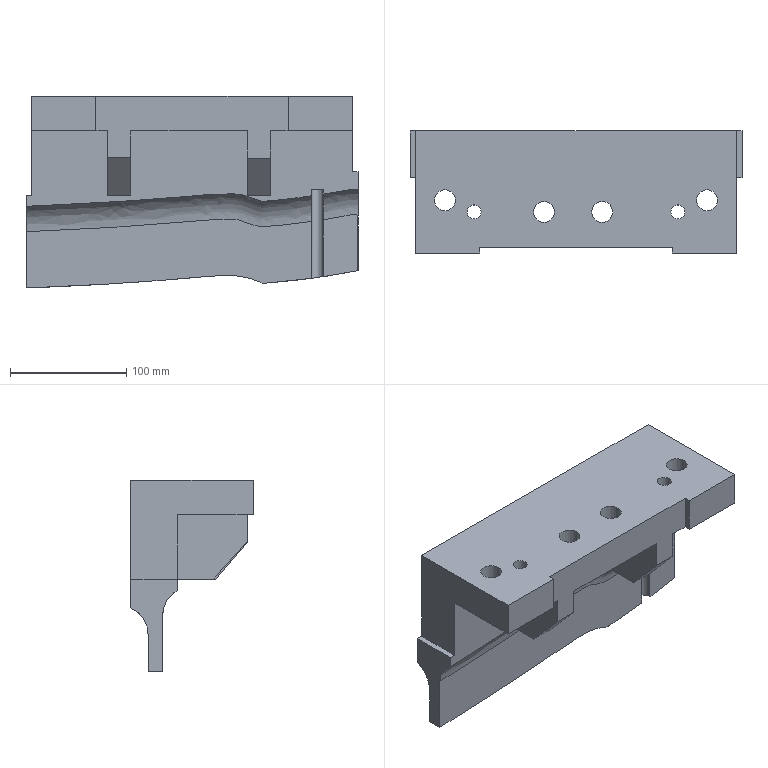Part | NX | features solid 2 | 1 solid | 61 faces | box 285.798 x 105 x 164.785 mm | volume 1866642 mm3 | plane 35 | spline 13 | cylinder 13 | commonest cylinder face diameters 18 x4 26 x4 12 x2 20 x2 10 x1